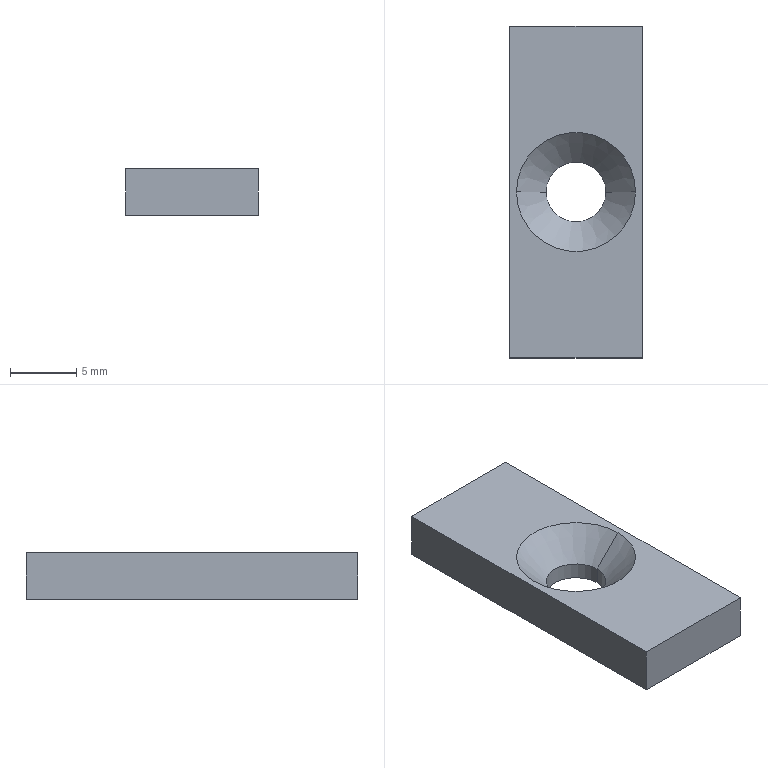Part | STEP file | 11-FG-E02811 | 1 solid | 10 faces | box 10 x 25 x 3.5 mm | volume 772.571 mm3 | plane 6 | cone 2 | cylinder 2 | commonest cylinder face diameters 4.5 x2
STEP:
#1=CARTESIAN_POINT('',(-2.25,0.,1.27));
#2=VERTEX_POINT('',#1);
#3=CARTESIAN_POINT('',(2.25,0.,1.27));
#4=VERTEX_POINT('',#3);
#5=CARTESIAN_POINT('',(0.,0.,1.27));
#6=DIRECTION('',(0.,0.,1.));
#7=DIRECTION('',(1.,0.,0.));
#8=AXIS2_PLACEMENT_3D('',#5,#6,#7);
#9=CIRCLE('',#8,2.25);
#10=EDGE_CURVE('',#2,#4,#9,.T.);
#11=ORIENTED_EDGE('',*,*,#10,.F.);
#12=CARTESIAN_POINT('',(-4.48,0.,3.5));
#13=VERTEX_POINT('',#12);
#14=CARTESIAN_POINT('',(-4.48,0.,3.5));
#15=DIRECTION('',(-0.7071,0.,0.7071));
#16=VECTOR('',#15,1000.);
#17=LINE('',#14,#16);
#18=EDGE_CURVE('',#2,#13,#17,.T.);
#19=ORIENTED_EDGE('',*,*,#18,.T.);
#20=CARTESIAN_POINT('',(4.48,0.,3.5));
#21=VERTEX_POINT('',#20);
#22=CARTESIAN_POINT('',(0.,0.,3.5));
#23=DIRECTION('',(0.,0.,1.));
#24=DIRECTION('',(1.,0.,0.));
#25=AXIS2_PLACEMENT_3D('',#22,#23,#24);
#26=CIRCLE('',#25,4.48);
#27=EDGE_CURVE('',#13,#21,#26,.T.);
#28=ORIENTED_EDGE('',*,*,#27,.T.);
#29=CARTESIAN_POINT('',(4.48,0.,3.5));
#30=DIRECTION('',(0.7071,0.,0.7071));
#31=VECTOR('',#30,1000.);
#32=LINE('',#29,#31);
#33=EDGE_CURVE('',#4,#21,#32,.T.);
#34=ORIENTED_EDGE('',*,*,#33,.F.);
#35=EDGE_LOOP('',(#11,#19,#28,#34));
#36=FACE_OUTER_BOUND('',#35,.T.);
#37=CARTESIAN_POINT('',(0.,0.,3.5));
#38=DIRECTION('',(0.,0.,1.));
#39=DIRECTION('',(1.,0.,0.));
#40=AXIS2_PLACEMENT_3D('',#37,#38,#39);
#41=CONICAL_SURFACE('',#40,4.48,0.7854);
#42=ADVANCED_FACE('',(#36),#41,.F.);
#43=CARTESIAN_POINT('',(-2.25,0.,0.));
#44=VERTEX_POINT('',#43);
#45=CARTESIAN_POINT('',(2.25,0.,0.));
#46=VERTEX_POINT('',#45);
#47=CARTESIAN_POINT('',(0.,0.,0.));
#48=DIRECTION('',(0.,0.,1.));
#49=DIRECTION('',(1.,0.,0.));
#50=AXIS2_PLACEMENT_3D('',#47,#48,#49);
#51=CIRCLE('',#50,2.25);
#52=EDGE_CURVE('',#44,#46,#51,.T.);
#53=ORIENTED_EDGE('',*,*,#52,.F.);
#54=CARTESIAN_POINT('',(-2.25,0.,3.5));
#55=DIRECTION('',(0.,0.,1.));
#56=VECTOR('',#55,1000.);
#57=LINE('',#54,#56);
#58=EDGE_CURVE('',#44,#2,#57,.T.);
#59=ORIENTED_EDGE('',*,*,#58,.T.);
#60=ORIENTED_EDGE('',*,*,#10,.T.);
#61=CARTESIAN_POINT('',(2.25,0.,3.5));
#62=DIRECTION('',(0.,0.,1.));
#63=VECTOR('',#62,1000.);
#64=LINE('',#61,#63);
#65=EDGE_CURVE('',#46,#4,#64,.T.);
#66=ORIENTED_EDGE('',*,*,#65,.F.);
#67=EDGE_LOOP('',(#53,#59,#60,#66));
#68=FACE_OUTER_BOUND('',#67,.T.);
#69=CARTESIAN_POINT('',(0.,0.,3.5));
#70=DIRECTION('',(0.,0.,1.));
#71=DIRECTION('',(1.,0.,0.));
#72=AXIS2_PLACEMENT_3D('',#69,#70,#71);
#73=CYLINDRICAL_SURFACE('',#72,2.25);
#74=ADVANCED_FACE('',(#68),#73,.F.);
#75=CARTESIAN_POINT('',(5.,-12.5,0.));
#76=VERTEX_POINT('',#75);
#77=CARTESIAN_POINT('',(5.,12.5,0.));
#78=VERTEX_POINT('',#77);
#79=CARTESIAN_POINT('',(5.,12.5,0.));
#80=DIRECTION('',(0.,1.,0.));
#81=VECTOR('',#80,1000.);
#82=LINE('',#79,#81);
#83=EDGE_CURVE('',#76,#78,#82,.T.);
#84=ORIENTED_EDGE('',*,*,#83,.T.);
#85=CARTESIAN_POINT('',(5.,12.5,3.5));
#86=VERTEX_POINT('',#85);
#87=CARTESIAN_POINT('',(5.,12.5,3.5));
#88=DIRECTION('',(0.,0.,-1.));
#89=VECTOR('',#88,1000.);
#90=LINE('',#87,#89);
#91=EDGE_CURVE('',#86,#78,#90,.T.);
#92=ORIENTED_EDGE('',*,*,#91,.F.);
#93=CARTESIAN_POINT('',(5.,-12.5,3.5));
#94=VERTEX_POINT('',#93);
#95=CARTESIAN_POINT('',(5.,12.5,3.5));
#96=DIRECTION('',(0.,1.,0.));
#97=VECTOR('',#96,1000.);
#98=LINE('',#95,#97);
#99=EDGE_CURVE('',#94,#86,#98,.T.);
#100=ORIENTED_EDGE('',*,*,#99,.F.);
#101=CARTESIAN_POINT('',(5.,-12.5,3.5));
#102=DIRECTION('',(0.,0.,-1.));
#103=VECTOR('',#102,1000.);
#104=LINE('',#101,#103);
#105=EDGE_CURVE('',#94,#76,#104,.T.);
#106=ORIENTED_EDGE('',*,*,#105,.T.);
#107=EDGE_LOOP('',(#84,#92,#100,#106));
#108=FACE_OUTER_BOUND('',#107,.T.);
#109=CARTESIAN_POINT('',(5.,12.5,3.5));
#110=DIRECTION('',(-1.,0.,0.));
#111=DIRECTION('',(0.,0.,1.));
#112=AXIS2_PLACEMENT_3D('',#109,#110,#111);
#113=PLANE('',#112);
#114=ADVANCED_FACE('',(#108),#113,.F.);
#115=CARTESIAN_POINT('',(-5.,12.5,0.));
#116=VERTEX_POINT('',#115);
#117=CARTESIAN_POINT('',(-5.,12.5,0.));
#118=DIRECTION('',(-1.,0.,0.));
#119=VECTOR('',#118,1000.);
#120=LINE('',#117,#119);
#121=EDGE_CURVE('',#78,#116,#120,.T.);
#122=ORIENTED_EDGE('',*,*,#121,.T.);
#123=CARTESIAN_POINT('',(-5.,12.5,3.5));
#124=VERTEX_POINT('',#123);
#125=CARTESIAN_POINT('',(-5.,12.5,3.5));
#126=DIRECTION('',(0.,0.,-1.));
#127=VECTOR('',#126,1000.);
#128=LINE('',#125,#127);
#129=EDGE_CURVE('',#124,#116,#128,.T.);
#130=ORIENTED_EDGE('',*,*,#129,.F.);
#131=CARTESIAN_POINT('',(-5.,12.5,3.5));
#132=DIRECTION('',(-1.,0.,0.));
#133=VECTOR('',#132,1000.);
#134=LINE('',#131,#133);
#135=EDGE_CURVE('',#86,#124,#134,.T.);
#136=ORIENTED_EDGE('',*,*,#135,.F.);
#137=ORIENTED_EDGE('',*,*,#91,.T.);
#138=EDGE_LOOP('',(#122,#130,#136,#137));
#139=FACE_OUTER_BOUND('',#138,.T.);
#140=CARTESIAN_POINT('',(-5.,12.5,3.5));
#141=DIRECTION('',(0.,-1.,0.));
#142=DIRECTION('',(0.,0.,-1.));
#143=AXIS2_PLACEMENT_3D('',#140,#141,#142);
#144=PLANE('',#143);
#145=ADVANCED_FACE('',(#139),#144,.F.);
#146=CARTESIAN_POINT('',(-5.,-12.5,0.));
#147=VERTEX_POINT('',#146);
#148=CARTESIAN_POINT('',(-5.,12.5,0.));
#149=DIRECTION('',(0.,-1.,0.));
#150=VECTOR('',#149,1000.);
#151=LINE('',#148,#150);
#152=EDGE_CURVE('',#116,#147,#151,.T.);
#153=ORIENTED_EDGE('',*,*,#152,.T.);
#154=CARTESIAN_POINT('',(-5.,-12.5,3.5));
#155=VERTEX_POINT('',#154);
#156=CARTESIAN_POINT('',(-5.,-12.5,3.5));
#157=DIRECTION('',(0.,0.,-1.));
#158=VECTOR('',#157,1000.);
#159=LINE('',#156,#158);
#160=EDGE_CURVE('',#155,#147,#159,.T.);
#161=ORIENTED_EDGE('',*,*,#160,.F.);
#162=CARTESIAN_POINT('',(-5.,12.5,3.5));
#163=DIRECTION('',(0.,-1.,0.));
#164=VECTOR('',#163,1000.);
#165=LINE('',#162,#164);
#166=EDGE_CURVE('',#124,#155,#165,.T.);
#167=ORIENTED_EDGE('',*,*,#166,.F.);
#168=ORIENTED_EDGE('',*,*,#129,.T.);
#169=EDGE_LOOP('',(#153,#161,#167,#168));
#170=FACE_OUTER_BOUND('',#169,.T.);
#171=CARTESIAN_POINT('',(-5.,12.5,3.5));
#172=DIRECTION('',(1.,0.,0.));
#173=DIRECTION('',(0.,0.,-1.));
#174=AXIS2_PLACEMENT_3D('',#171,#172,#173);
#175=PLANE('',#174);
#176=ADVANCED_FACE('',(#170),#175,.F.);
#177=CARTESIAN_POINT('',(-5.,-12.5,0.));
#178=DIRECTION('',(1.,0.,0.));
#179=VECTOR('',#178,1000.);
#180=LINE('',#177,#179);
#181=EDGE_CURVE('',#147,#76,#180,.T.);
#182=ORIENTED_EDGE('',*,*,#181,.T.);
#183=ORIENTED_EDGE('',*,*,#105,.F.);
#184=CARTESIAN_POINT('',(-5.,-12.5,3.5));
#185=DIRECTION('',(1.,0.,0.));
#186=VECTOR('',#185,1000.);
#187=LINE('',#184,#186);
#188=EDGE_CURVE('',#155,#94,#187,.T.);
#189=ORIENTED_EDGE('',*,*,#188,.F.);
#190=ORIENTED_EDGE('',*,*,#160,.T.);
#191=EDGE_LOOP('',(#182,#183,#189,#190));
#192=FACE_OUTER_BOUND('',#191,.T.);
#193=CARTESIAN_POINT('',(-5.,-12.5,3.5));
#194=DIRECTION('',(0.,1.,0.));
#195=DIRECTION('',(0.,0.,1.));
#196=AXIS2_PLACEMENT_3D('',#193,#194,#195);
#197=PLANE('',#196);
#198=ADVANCED_FACE('',(#192),#197,.F.);
#199=CARTESIAN_POINT('',(0.,0.,3.5));
#200=DIRECTION('',(0.,0.,1.));
#201=DIRECTION('',(1.,0.,0.));
#202=AXIS2_PLACEMENT_3D('',#199,#200,#201);
#203=CIRCLE('',#202,4.48);
#204=EDGE_CURVE('',#21,#13,#203,.T.);
#205=ORIENTED_EDGE('',*,*,#204,.F.);
#206=ORIENTED_EDGE('',*,*,#27,.F.);
#207=EDGE_LOOP('',(#205,#206));
#208=FACE_BOUND('',#207,.T.);
#209=ORIENTED_EDGE('',*,*,#99,.T.);
#210=ORIENTED_EDGE('',*,*,#135,.T.);
#211=ORIENTED_EDGE('',*,*,#166,.T.);
#212=ORIENTED_EDGE('',*,*,#188,.T.);
#213=EDGE_LOOP('',(#209,#210,#211,#212));
#214=FACE_OUTER_BOUND('',#213,.T.);
#215=CARTESIAN_POINT('',(0.,0.,3.5));
#216=DIRECTION('',(0.,0.,1.));
#217=DIRECTION('',(1.,0.,0.));
#218=AXIS2_PLACEMENT_3D('',#215,#216,#217);
#219=PLANE('',#218);
#220=ADVANCED_FACE('',(#208,#214),#219,.T.);
#221=CARTESIAN_POINT('',(0.,0.,0.));
#222=DIRECTION('',(0.,0.,1.));
#223=DIRECTION('',(1.,0.,0.));
#224=AXIS2_PLACEMENT_3D('',#221,#222,#223);
#225=CIRCLE('',#224,2.25);
#226=EDGE_CURVE('',#46,#44,#225,.T.);
#227=ORIENTED_EDGE('',*,*,#226,.T.);
#228=ORIENTED_EDGE('',*,*,#52,.T.);
#229=EDGE_LOOP('',(#227,#228));
#230=FACE_BOUND('',#229,.T.);
#231=ORIENTED_EDGE('',*,*,#83,.F.);
#232=ORIENTED_EDGE('',*,*,#181,.F.);
#233=ORIENTED_EDGE('',*,*,#152,.F.);
#234=ORIENTED_EDGE('',*,*,#121,.F.);
#235=EDGE_LOOP('',(#231,#232,#233,#234));
#236=FACE_OUTER_BOUND('',#235,.T.);
#237=CARTESIAN_POINT('',(0.,0.,0.));
#238=DIRECTION('',(0.,0.,1.));
#239=DIRECTION('',(1.,0.,0.));
#240=AXIS2_PLACEMENT_3D('',#237,#238,#239);
#241=PLANE('',#240);
#242=ADVANCED_FACE('',(#230,#236),#241,.F.);
#243=ORIENTED_EDGE('',*,*,#58,.F.);
#244=ORIENTED_EDGE('',*,*,#226,.F.);
#245=ORIENTED_EDGE('',*,*,#65,.T.);
#246=CARTESIAN_POINT('',(0.,0.,1.27));
#247=DIRECTION('',(0.,0.,1.));
#248=DIRECTION('',(1.,0.,0.));
#249=AXIS2_PLACEMENT_3D('',#246,#247,#248);
#250=CIRCLE('',#249,2.25);
#251=EDGE_CURVE('',#4,#2,#250,.T.);
#252=ORIENTED_EDGE('',*,*,#251,.T.);
#253=EDGE_LOOP('',(#243,#244,#245,#252));
#254=FACE_OUTER_BOUND('',#253,.T.);
#255=CARTESIAN_POINT('',(0.,0.,3.5));
#256=DIRECTION('',(0.,0.,1.));
#257=DIRECTION('',(1.,0.,0.));
#258=AXIS2_PLACEMENT_3D('',#255,#256,#257);
#259=CYLINDRICAL_SURFACE('',#258,2.25);
#260=ADVANCED_FACE('',(#254),#259,.F.);
#261=ORIENTED_EDGE('',*,*,#18,.F.);
#262=ORIENTED_EDGE('',*,*,#251,.F.);
#263=ORIENTED_EDGE('',*,*,#33,.T.);
#264=ORIENTED_EDGE('',*,*,#204,.T.);
#265=EDGE_LOOP('',(#261,#262,#263,#264));
#266=FACE_OUTER_BOUND('',#265,.T.);
#267=CARTESIAN_POINT('',(0.,0.,3.5));
#268=DIRECTION('',(0.,0.,1.));
#269=DIRECTION('',(1.,0.,0.));
#270=AXIS2_PLACEMENT_3D('',#267,#268,#269);
#271=CONICAL_SURFACE('',#270,4.48,0.7854);
#272=ADVANCED_FACE('',(#266),#271,.F.);
#273=CLOSED_SHELL('',(#42,#74,#114,#145,#176,#198,#220,#242,#260,#272));
#274=MANIFOLD_SOLID_BREP('',#273);
#275=CARTESIAN_POINT('',(0.,0.,0.));
#276=DIRECTION('',(0.,0.,1.));
#277=DIRECTION('',(1.,0.,0.));
#278=AXIS2_PLACEMENT_3D('',#275,#276,#277);
#279=(LENGTH_UNIT()NAMED_UNIT(*)SI_UNIT(.MILLI.,.METRE.));
#280=UNCERTAINTY_MEASURE_WITH_UNIT(LENGTH_MEASURE(0.00001),#279,'','');
#281=(NAMED_UNIT(*)PLANE_ANGLE_UNIT()SI_UNIT($,.RADIAN.));
#282=(NAMED_UNIT(*)SI_UNIT($,.STERADIAN.)SOLID_ANGLE_UNIT());
#283=(GEOMETRIC_REPRESENTATION_CONTEXT(3)GLOBAL_UNCERTAINTY_ASSIGNED_CONTEXT((#280))GLOBAL_UNIT_ASSIGNED_CONTEXT((#279,#281,#282))REPRESENTATION_CONTEXT('',''));
#284=ADVANCED_BREP_SHAPE_REPRESENTATION('',(#274,#278),#283);